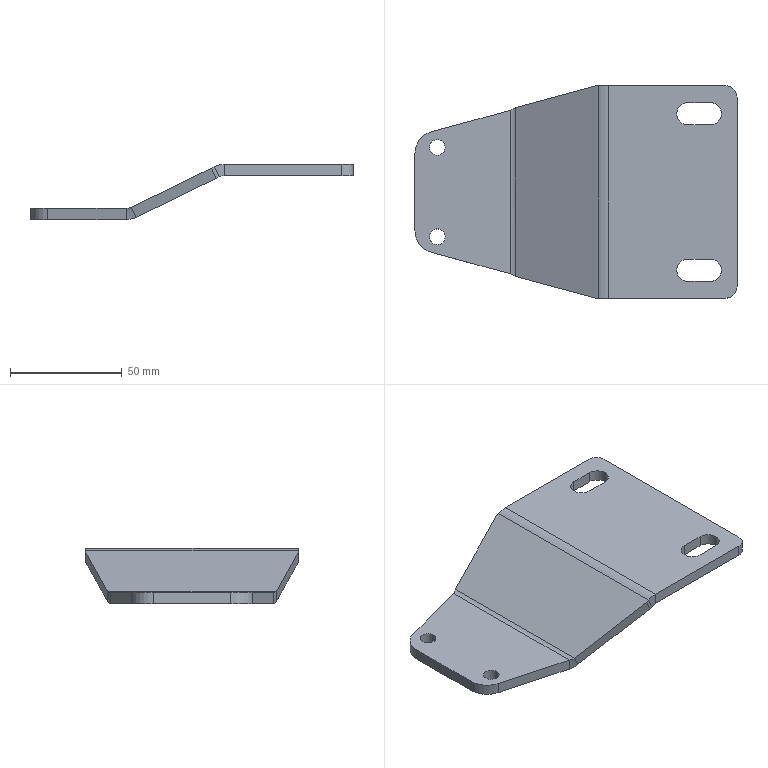Part | STEP file | SYL_0392D6J1SYL0380DJ10-1504831 | 1 solid | 44 faces | box 144.153 x 95 x 24.659 mm | volume 58803 mm3 | plane 22 | cylinder 20 | spline 2 | commonest cylinder face diameters 10 x12 7 x4 20 x4
STEP:
#1=CARTESIAN_POINT('',(18.,30.,0.));
#2=VERTEX_POINT('',#1);
#3=CARTESIAN_POINT('',(18.,30.,5.));
#4=VERTEX_POINT('',#3);
#5=CARTESIAN_POINT('',(18.,30.,5.));
#6=DIRECTION('',(0.,0.,1.));
#7=VECTOR('',#6,1000.);
#8=LINE('',#5,#7);
#9=EDGE_CURVE('',#2,#4,#8,.T.);
#10=ORIENTED_EDGE('',*,*,#9,.F.);
#11=CARTESIAN_POINT('',(8.,30.,0.));
#12=VERTEX_POINT('',#11);
#13=CARTESIAN_POINT('',(0.,30.,0.));
#14=DIRECTION('',(1.,0.,0.));
#15=VECTOR('',#14,1000.);
#16=LINE('',#13,#15);
#17=EDGE_CURVE('',#12,#2,#16,.T.);
#18=ORIENTED_EDGE('',*,*,#17,.F.);
#19=CARTESIAN_POINT('',(8.,30.,5.));
#20=VERTEX_POINT('',#19);
#21=CARTESIAN_POINT('',(8.,30.,5.));
#22=DIRECTION('',(0.,0.,1.));
#23=VECTOR('',#22,1000.);
#24=LINE('',#21,#23);
#25=EDGE_CURVE('',#12,#20,#24,.T.);
#26=ORIENTED_EDGE('',*,*,#25,.T.);
#27=CARTESIAN_POINT('',(8.,30.,5.));
#28=DIRECTION('',(1.,0.,0.));
#29=VECTOR('',#28,1000.);
#30=LINE('',#27,#29);
#31=EDGE_CURVE('',#20,#4,#30,.T.);
#32=ORIENTED_EDGE('',*,*,#31,.T.);
#33=EDGE_LOOP('',(#10,#18,#26,#32));
#34=FACE_OUTER_BOUND('',#33,.T.);
#35=CARTESIAN_POINT('',(8.,30.,5.));
#36=DIRECTION('',(0.,-1.,0.));
#37=DIRECTION('',(1.,0.,0.));
#38=AXIS2_PLACEMENT_3D('',#35,#36,#37);
#39=PLANE('',#38);
#40=ADVANCED_FACE('',(#34),#39,.F.);
#41=ORIENTED_EDGE('',*,*,#25,.F.);
#42=CARTESIAN_POINT('',(3.,35.,0.));
#43=VERTEX_POINT('',#42);
#44=CARTESIAN_POINT('',(8.,35.,0.));
#45=DIRECTION('',(0.,0.,-1.));
#46=DIRECTION('',(-1.,0.,0.));
#47=AXIS2_PLACEMENT_3D('',#44,#45,#46);
#48=CIRCLE('',#47,5.);
#49=EDGE_CURVE('',#12,#43,#48,.T.);
#50=ORIENTED_EDGE('',*,*,#49,.T.);
#51=CARTESIAN_POINT('',(3.,35.,5.));
#52=VERTEX_POINT('',#51);
#53=CARTESIAN_POINT('',(3.,35.,5.));
#54=DIRECTION('',(0.,0.,1.));
#55=VECTOR('',#54,1000.);
#56=LINE('',#53,#55);
#57=EDGE_CURVE('',#43,#52,#56,.T.);
#58=ORIENTED_EDGE('',*,*,#57,.T.);
#59=CARTESIAN_POINT('',(8.,35.,5.));
#60=DIRECTION('',(0.,0.,-1.));
#61=DIRECTION('',(0.,-1.,0.));
#62=AXIS2_PLACEMENT_3D('',#59,#60,#61);
#63=CIRCLE('',#62,5.);
#64=EDGE_CURVE('',#20,#52,#63,.T.);
#65=ORIENTED_EDGE('',*,*,#64,.F.);
#66=EDGE_LOOP('',(#41,#50,#58,#65));
#67=FACE_OUTER_BOUND('',#66,.T.);
#68=CARTESIAN_POINT('',(8.,35.,5.));
#69=DIRECTION('',(0.,0.,1.));
#70=DIRECTION('',(1.,0.,0.));
#71=AXIS2_PLACEMENT_3D('',#68,#69,#70);
#72=CYLINDRICAL_SURFACE('',#71,5.);
#73=ADVANCED_FACE('',(#67),#72,.F.);
#74=ORIENTED_EDGE('',*,*,#57,.F.);
#75=CARTESIAN_POINT('',(8.,40.,0.));
#76=VERTEX_POINT('',#75);
#77=CARTESIAN_POINT('',(8.,35.,0.));
#78=DIRECTION('',(0.,0.,-1.));
#79=DIRECTION('',(-1.,0.,0.));
#80=AXIS2_PLACEMENT_3D('',#77,#78,#79);
#81=CIRCLE('',#80,5.);
#82=EDGE_CURVE('',#43,#76,#81,.T.);
#83=ORIENTED_EDGE('',*,*,#82,.T.);
#84=CARTESIAN_POINT('',(8.,40.,5.));
#85=VERTEX_POINT('',#84);
#86=CARTESIAN_POINT('',(8.,40.,5.));
#87=DIRECTION('',(0.,0.,1.));
#88=VECTOR('',#87,1000.);
#89=LINE('',#86,#88);
#90=EDGE_CURVE('',#76,#85,#89,.T.);
#91=ORIENTED_EDGE('',*,*,#90,.T.);
#92=CARTESIAN_POINT('',(8.,35.,5.));
#93=DIRECTION('',(0.,0.,-1.));
#94=DIRECTION('',(-1.,0.,0.));
#95=AXIS2_PLACEMENT_3D('',#92,#93,#94);
#96=CIRCLE('',#95,5.);
#97=EDGE_CURVE('',#52,#85,#96,.T.);
#98=ORIENTED_EDGE('',*,*,#97,.F.);
#99=EDGE_LOOP('',(#74,#83,#91,#98));
#100=FACE_OUTER_BOUND('',#99,.T.);
#101=CARTESIAN_POINT('',(8.,35.,5.));
#102=DIRECTION('',(0.,0.,1.));
#103=DIRECTION('',(1.,0.,0.));
#104=AXIS2_PLACEMENT_3D('',#101,#102,#103);
#105=CYLINDRICAL_SURFACE('',#104,5.);
#106=ADVANCED_FACE('',(#100),#105,.F.);
#107=ORIENTED_EDGE('',*,*,#90,.F.);
#108=CARTESIAN_POINT('',(18.,40.,0.));
#109=VERTEX_POINT('',#108);
#110=CARTESIAN_POINT('',(0.,40.,0.));
#111=DIRECTION('',(-1.,0.,0.));
#112=VECTOR('',#111,1000.);
#113=LINE('',#110,#112);
#114=EDGE_CURVE('',#109,#76,#113,.T.);
#115=ORIENTED_EDGE('',*,*,#114,.F.);
#116=CARTESIAN_POINT('',(18.,40.,5.));
#117=VERTEX_POINT('',#116);
#118=CARTESIAN_POINT('',(18.,40.,5.));
#119=DIRECTION('',(0.,0.,1.));
#120=VECTOR('',#119,1000.);
#121=LINE('',#118,#120);
#122=EDGE_CURVE('',#109,#117,#121,.T.);
#123=ORIENTED_EDGE('',*,*,#122,.T.);
#124=CARTESIAN_POINT('',(18.,40.,5.));
#125=DIRECTION('',(-1.,0.,0.));
#126=VECTOR('',#125,1000.);
#127=LINE('',#124,#126);
#128=EDGE_CURVE('',#117,#85,#127,.T.);
#129=ORIENTED_EDGE('',*,*,#128,.T.);
#130=EDGE_LOOP('',(#107,#115,#123,#129));
#131=FACE_OUTER_BOUND('',#130,.T.);
#132=CARTESIAN_POINT('',(18.,40.,5.));
#133=DIRECTION('',(0.,1.,0.));
#134=DIRECTION('',(-1.,0.,0.));
#135=AXIS2_PLACEMENT_3D('',#132,#133,#134);
#136=PLANE('',#135);
#137=ADVANCED_FACE('',(#131),#136,.F.);
#138=ORIENTED_EDGE('',*,*,#122,.F.);
#139=CARTESIAN_POINT('',(23.,35.,0.));
#140=VERTEX_POINT('',#139);
#141=CARTESIAN_POINT('',(18.,35.,0.));
#142=DIRECTION('',(0.,0.,-1.));
#143=DIRECTION('',(-1.,0.,0.));
#144=AXIS2_PLACEMENT_3D('',#141,#142,#143);
#145=CIRCLE('',#144,5.);
#146=EDGE_CURVE('',#109,#140,#145,.T.);
#147=ORIENTED_EDGE('',*,*,#146,.T.);
#148=CARTESIAN_POINT('',(23.,35.,5.));
#149=VERTEX_POINT('',#148);
#150=CARTESIAN_POINT('',(23.,35.,5.));
#151=DIRECTION('',(0.,0.,1.));
#152=VECTOR('',#151,1000.);
#153=LINE('',#150,#152);
#154=EDGE_CURVE('',#140,#149,#153,.T.);
#155=ORIENTED_EDGE('',*,*,#154,.T.);
#156=CARTESIAN_POINT('',(18.,35.,5.));
#157=DIRECTION('',(0.,0.,-1.));
#158=DIRECTION('',(0.,1.,0.));
#159=AXIS2_PLACEMENT_3D('',#156,#157,#158);
#160=CIRCLE('',#159,5.);
#161=EDGE_CURVE('',#117,#149,#160,.T.);
#162=ORIENTED_EDGE('',*,*,#161,.F.);
#163=EDGE_LOOP('',(#138,#147,#155,#162));
#164=FACE_OUTER_BOUND('',#163,.T.);
#165=CARTESIAN_POINT('',(18.,35.,5.));
#166=DIRECTION('',(0.,0.,1.));
#167=DIRECTION('',(1.,0.,0.));
#168=AXIS2_PLACEMENT_3D('',#165,#166,#167);
#169=CYLINDRICAL_SURFACE('',#168,5.);
#170=ADVANCED_FACE('',(#164),#169,.F.);
#171=CARTESIAN_POINT('',(8.,-40.,0.));
#172=VERTEX_POINT('',#171);
#173=CARTESIAN_POINT('',(8.,-40.,5.));
#174=VERTEX_POINT('',#173);
#175=CARTESIAN_POINT('',(8.,-40.,5.));
#176=DIRECTION('',(0.,0.,1.));
#177=VECTOR('',#176,1000.);
#178=LINE('',#175,#177);
#179=EDGE_CURVE('',#172,#174,#178,.T.);
#180=ORIENTED_EDGE('',*,*,#179,.F.);
#181=CARTESIAN_POINT('',(3.,-35.,0.));
#182=VERTEX_POINT('',#181);
#183=CARTESIAN_POINT('',(8.,-35.,0.));
#184=DIRECTION('',(0.,0.,-1.));
#185=DIRECTION('',(-1.,0.,0.));
#186=AXIS2_PLACEMENT_3D('',#183,#184,#185);
#187=CIRCLE('',#186,5.);
#188=EDGE_CURVE('',#172,#182,#187,.T.);
#189=ORIENTED_EDGE('',*,*,#188,.T.);
#190=CARTESIAN_POINT('',(3.,-35.,5.));
#191=VERTEX_POINT('',#190);
#192=CARTESIAN_POINT('',(3.,-35.,5.));
#193=DIRECTION('',(0.,0.,1.));
#194=VECTOR('',#193,1000.);
#195=LINE('',#192,#194);
#196=EDGE_CURVE('',#182,#191,#195,.T.);
#197=ORIENTED_EDGE('',*,*,#196,.T.);
#198=CARTESIAN_POINT('',(8.,-35.,5.));
#199=DIRECTION('',(0.,0.,-1.));
#200=DIRECTION('',(0.,-1.,0.));
#201=AXIS2_PLACEMENT_3D('',#198,#199,#200);
#202=CIRCLE('',#201,5.);
#203=EDGE_CURVE('',#174,#191,#202,.T.);
#204=ORIENTED_EDGE('',*,*,#203,.F.);
#205=EDGE_LOOP('',(#180,#189,#197,#204));
#206=FACE_OUTER_BOUND('',#205,.T.);
#207=CARTESIAN_POINT('',(8.,-35.,5.));
#208=DIRECTION('',(0.,0.,1.));
#209=DIRECTION('',(1.,0.,0.));
#210=AXIS2_PLACEMENT_3D('',#207,#208,#209);
#211=CYLINDRICAL_SURFACE('',#210,5.);
#212=ADVANCED_FACE('',(#206),#211,.F.);
#213=ORIENTED_EDGE('',*,*,#196,.F.);
#214=CARTESIAN_POINT('',(8.,-30.,0.));
#215=VERTEX_POINT('',#214);
#216=CARTESIAN_POINT('',(8.,-35.,0.));
#217=DIRECTION('',(0.,0.,-1.));
#218=DIRECTION('',(-1.,0.,0.));
#219=AXIS2_PLACEMENT_3D('',#216,#217,#218);
#220=CIRCLE('',#219,5.);
#221=EDGE_CURVE('',#182,#215,#220,.T.);
#222=ORIENTED_EDGE('',*,*,#221,.T.);
#223=CARTESIAN_POINT('',(8.,-30.,5.));
#224=VERTEX_POINT('',#223);
#225=CARTESIAN_POINT('',(8.,-30.,5.));
#226=DIRECTION('',(0.,0.,1.));
#227=VECTOR('',#226,1000.);
#228=LINE('',#225,#227);
#229=EDGE_CURVE('',#215,#224,#228,.T.);
#230=ORIENTED_EDGE('',*,*,#229,.T.);
#231=CARTESIAN_POINT('',(8.,-35.,5.));
#232=DIRECTION('',(0.,0.,-1.));
#233=DIRECTION('',(-1.,0.,0.));
#234=AXIS2_PLACEMENT_3D('',#231,#232,#233);
#235=CIRCLE('',#234,5.);
#236=EDGE_CURVE('',#191,#224,#235,.T.);
#237=ORIENTED_EDGE('',*,*,#236,.F.);
#238=EDGE_LOOP('',(#213,#222,#230,#237));
#239=FACE_OUTER_BOUND('',#238,.T.);
#240=CARTESIAN_POINT('',(8.,-35.,5.));
#241=DIRECTION('',(0.,0.,1.));
#242=DIRECTION('',(1.,0.,0.));
#243=AXIS2_PLACEMENT_3D('',#240,#241,#242);
#244=CYLINDRICAL_SURFACE('',#243,5.);
#245=ADVANCED_FACE('',(#239),#244,.F.);
#246=ORIENTED_EDGE('',*,*,#229,.F.);
#247=CARTESIAN_POINT('',(18.,-30.,0.));
#248=VERTEX_POINT('',#247);
#249=CARTESIAN_POINT('',(0.,-30.,0.));
#250=DIRECTION('',(-1.,0.,0.));
#251=VECTOR('',#250,1000.);
#252=LINE('',#249,#251);
#253=EDGE_CURVE('',#248,#215,#252,.T.);
#254=ORIENTED_EDGE('',*,*,#253,.F.);
#255=CARTESIAN_POINT('',(18.,-30.,5.));
#256=VERTEX_POINT('',#255);
#257=CARTESIAN_POINT('',(18.,-30.,5.));
#258=DIRECTION('',(0.,0.,1.));
#259=VECTOR('',#258,1000.);
#260=LINE('',#257,#259);
#261=EDGE_CURVE('',#248,#256,#260,.T.);
#262=ORIENTED_EDGE('',*,*,#261,.T.);
#263=CARTESIAN_POINT('',(18.,-30.,5.));
#264=DIRECTION('',(-1.,0.,0.));
#265=VECTOR('',#264,1000.);
#266=LINE('',#263,#265);
#267=EDGE_CURVE('',#256,#224,#266,.T.);
#268=ORIENTED_EDGE('',*,*,#267,.T.);
#269=EDGE_LOOP('',(#246,#254,#262,#268));
#270=FACE_OUTER_BOUND('',#269,.T.);
#271=CARTESIAN_POINT('',(18.,-30.,5.));
#272=DIRECTION('',(0.,1.,0.));
#273=DIRECTION('',(-1.,0.,0.));
#274=AXIS2_PLACEMENT_3D('',#271,#272,#273);
#275=PLANE('',#274);
#276=ADVANCED_FACE('',(#270),#275,.F.);
#277=ORIENTED_EDGE('',*,*,#261,.F.);
#278=CARTESIAN_POINT('',(23.,-35.,0.));
#279=VERTEX_POINT('',#278);
#280=CARTESIAN_POINT('',(18.,-35.,0.));
#281=DIRECTION('',(0.,0.,-1.));
#282=DIRECTION('',(-1.,0.,0.));
#283=AXIS2_PLACEMENT_3D('',#280,#281,#282);
#284=CIRCLE('',#283,5.);
#285=EDGE_CURVE('',#248,#279,#284,.T.);
#286=ORIENTED_EDGE('',*,*,#285,.T.);
#287=CARTESIAN_POINT('',(23.,-35.,5.));
#288=VERTEX_POINT('',#287);
#289=CARTESIAN_POINT('',(23.,-35.,5.));
#290=DIRECTION('',(0.,0.,1.));
#291=VECTOR('',#290,1000.);
#292=LINE('',#289,#291);
#293=EDGE_CURVE('',#279,#288,#292,.T.);
#294=ORIENTED_EDGE('',*,*,#293,.T.);
#295=CARTESIAN_POINT('',(18.,-35.,5.));
#296=DIRECTION('',(0.,0.,-1.));
#297=DIRECTION('',(0.,1.,0.));
#298=AXIS2_PLACEMENT_3D('',#295,#296,#297);
#299=CIRCLE('',#298,5.);
#300=EDGE_CURVE('',#256,#288,#299,.T.);
#301=ORIENTED_EDGE('',*,*,#300,.F.);
#302=EDGE_LOOP('',(#277,#286,#294,#301));
#303=FACE_OUTER_BOUND('',#302,.T.);
#304=CARTESIAN_POINT('',(18.,-35.,5.));
#305=DIRECTION('',(0.,0.,1.));
#306=DIRECTION('',(1.,0.,0.));
#307=AXIS2_PLACEMENT_3D('',#304,#305,#306);
#308=CYLINDRICAL_SURFACE('',#307,5.);
#309=ADVANCED_FACE('',(#303),#308,.F.);
#310=ORIENTED_EDGE('',*,*,#293,.F.);
#311=CARTESIAN_POINT('',(18.,-40.,0.));
#312=VERTEX_POINT('',#311);
#313=CARTESIAN_POINT('',(18.,-35.,0.));
#314=DIRECTION('',(0.,0.,-1.));
#315=DIRECTION('',(-1.,0.,0.));
#316=AXIS2_PLACEMENT_3D('',#313,#314,#315);
#317=CIRCLE('',#316,5.);
#318=EDGE_CURVE('',#279,#312,#317,.T.);
#319=ORIENTED_EDGE('',*,*,#318,.T.);
#320=CARTESIAN_POINT('',(18.,-40.,5.));
#321=VERTEX_POINT('',#320);
#322=CARTESIAN_POINT('',(18.,-40.,5.));
#323=DIRECTION('',(0.,0.,1.));
#324=VECTOR('',#323,1000.);
#325=LINE('',#322,#324);
#326=EDGE_CURVE('',#312,#321,#325,.T.);
#327=ORIENTED_EDGE('',*,*,#326,.T.);
#328=CARTESIAN_POINT('',(18.,-35.,5.));
#329=DIRECTION('',(0.,0.,-1.));
#330=DIRECTION('',(1.,0.,0.));
#331=AXIS2_PLACEMENT_3D('',#328,#329,#330);
#332=CIRCLE('',#331,5.);
#333=EDGE_CURVE('',#288,#321,#332,.T.);
#334=ORIENTED_EDGE('',*,*,#333,.F.);
#335=EDGE_LOOP('',(#310,#319,#327,#334));
#336=FACE_OUTER_BOUND('',#335,.T.);
#337=CARTESIAN_POINT('',(18.,-35.,5.));
#338=DIRECTION('',(0.,0.,1.));
#339=DIRECTION('',(1.,0.,0.));
#340=AXIS2_PLACEMENT_3D('',#337,#338,#339);
#341=CYLINDRICAL_SURFACE('',#340,5.);
#342=ADVANCED_FACE('',(#336),#341,.F.);
#343=CARTESIAN_POINT('',(-100.653,-20.,-19.659));
#344=VERTEX_POINT('',#343);
#345=CARTESIAN_POINT('',(-100.653,-20.,-14.659));
#346=VERTEX_POINT('',#345);
#347=CARTESIAN_POINT('',(-100.653,-20.,-14.659));
#348=DIRECTION('',(0.,0.,1.));
#349=VECTOR('',#348,1000.);
#350=LINE('',#347,#349);
#351=EDGE_CURVE('',#344,#346,#350,.T.);
#352=ORIENTED_EDGE('',*,*,#351,.F.);
#353=CARTESIAN_POINT('',(-107.653,-20.,-19.659));
#354=VERTEX_POINT('',#353);
#355=CARTESIAN_POINT('',(-104.153,-20.,-19.659));
#356=DIRECTION('',(0.,0.,-1.));
#357=DIRECTION('',(-1.,0.,0.));
#358=AXIS2_PLACEMENT_3D('',#355,#356,#357);
#359=CIRCLE('',#358,3.5);
#360=EDGE_CURVE('',#344,#354,#359,.T.);
#361=ORIENTED_EDGE('',*,*,#360,.T.);
#362=CARTESIAN_POINT('',(-107.653,-20.,-14.659));
#363=VERTEX_POINT('',#362);
#364=CARTESIAN_POINT('',(-107.653,-20.,-14.659));
#365=DIRECTION('',(0.,0.,1.));
#366=VECTOR('',#365,1000.);
#367=LINE('',#364,#366);
#368=EDGE_CURVE('',#354,#363,#367,.T.);
#369=ORIENTED_EDGE('',*,*,#368,.T.);
#370=CARTESIAN_POINT('',(-104.153,-20.,-14.659));
#371=DIRECTION('',(0.,0.,-1.));
#372=DIRECTION('',(1.,0.,0.));
#373=AXIS2_PLACEMENT_3D('',#370,#371,#372);
#374=CIRCLE('',#373,3.5);
#375=EDGE_CURVE('',#346,#363,#374,.T.);
#376=ORIENTED_EDGE('',*,*,#375,.F.);
#377=EDGE_LOOP('',(#352,#361,#369,#376));
#378=FACE_OUTER_BOUND('',#377,.T.);
#379=CARTESIAN_POINT('',(-104.153,-20.,-14.659));
#380=DIRECTION('',(0.,0.,-1.));
#381=DIRECTION('',(-1.,0.,0.));
#382=AXIS2_PLACEMENT_3D('',#379,#380,#381);
#383=CYLINDRICAL_SURFACE('',#382,3.5);
#384=ADVANCED_FACE('',(#378),#383,.F.);
#385=CARTESIAN_POINT('',(-100.653,20.,-19.659));
#386=VERTEX_POINT('',#385);
#387=CARTESIAN_POINT('',(-100.653,20.,-14.659));
#388=VERTEX_POINT('',#387);
#389=CARTESIAN_POINT('',(-100.653,20.,-14.659));
#390=DIRECTION('',(0.,0.,1.));
#391=VECTOR('',#390,1000.);
#392=LINE('',#389,#391);
#393=EDGE_CURVE('',#386,#388,#392,.T.);
#394=ORIENTED_EDGE('',*,*,#393,.F.);
#395=CARTESIAN_POINT('',(-107.653,20.,-19.659));
#396=VERTEX_POINT('',#395);
#397=CARTESIAN_POINT('',(-104.153,20.,-19.659));
#398=DIRECTION('',(0.,0.,-1.));
#399=DIRECTION('',(-1.,0.,0.));
#400=AXIS2_PLACEMENT_3D('',#397,#398,#399);
#401=CIRCLE('',#400,3.5);
#402=EDGE_CURVE('',#386,#396,#401,.T.);
#403=ORIENTED_EDGE('',*,*,#402,.T.);
#404=CARTESIAN_POINT('',(-107.653,20.,-14.659));
#405=VERTEX_POINT('',#404);
#406=CARTESIAN_POINT('',(-107.653,20.,-14.659));
#407=DIRECTION('',(0.,0.,1.));
#408=VECTOR('',#407,1000.);
#409=LINE('',#406,#408);
#410=EDGE_CURVE('',#396,#405,#409,.T.);
#411=ORIENTED_EDGE('',*,*,#410,.T.);
#412=CARTESIAN_POINT('',(-104.153,20.,-14.659));
#413=DIRECTION('',(0.,0.,-1.));
#414=DIRECTION('',(1.,0.,0.));
#415=AXIS2_PLACEMENT_3D('',#412,#413,#414);
#416=CIRCLE('',#415,3.5);
#417=EDGE_CURVE('',#388,#405,#416,.T.);
#418=ORIENTED_EDGE('',*,*,#417,.F.);
#419=EDGE_LOOP('',(#394,#403,#411,#418));
#420=FACE_OUTER_BOUND('',#419,.T.);
#421=CARTESIAN_POINT('',(-104.153,20.,-14.659));
#422=DIRECTION('',(0.,0.,-1.));
#423=DIRECTION('',(-1.,0.,0.));
#424=AXIS2_PLACEMENT_3D('',#421,#422,#423);
#425=CYLINDRICAL_SURFACE('',#424,3.5);
#426=ADVANCED_FACE('',(#420),#425,.F.);
#427=CARTESIAN_POINT('',(-106.769,27.002,-19.659));
#428=VERTEX_POINT('',#427);
#429=CARTESIAN_POINT('',(-106.769,27.002,-14.659));
#430=VERTEX_POINT('',#429);
#431=CARTESIAN_POINT('',(-106.769,27.002,-14.659));
#432=DIRECTION('',(0.,0.,1.));
#433=VECTOR('',#432,1000.);
#434=LINE('',#431,#433);
#435=EDGE_CURVE('',#428,#430,#434,.T.);
#436=ORIENTED_EDGE('',*,*,#435,.F.);
#437=CARTESIAN_POINT('',(-114.153,17.35,-19.659));
#438=VERTEX_POINT('',#437);
#439=CARTESIAN_POINT('',(-104.153,17.35,-19.659));
#440=DIRECTION('',(0.,0.,1.));
#441=DIRECTION('',(1.,0.,0.));
#442=AXIS2_PLACEMENT_3D('',#439,#440,#441);
#443=CIRCLE('',#442,10.);
#444=EDGE_CURVE('',#428,#438,#443,.T.);
#445=ORIENTED_EDGE('',*,*,#444,.T.);
#446=CARTESIAN_POINT('',(-114.153,17.35,-14.659));
#447=VERTEX_POINT('',#446);
#448=CARTESIAN_POINT('',(-114.153,17.35,-14.659));
#449=DIRECTION('',(0.,0.,1.));
#450=VECTOR('',#449,1000.);
#451=LINE('',#448,#450);
#452=EDGE_CURVE('',#438,#447,#451,.T.);
#453=ORIENTED_EDGE('',*,*,#452,.T.);
#454=CARTESIAN_POINT('',(-104.153,17.35,-14.659));
#455=DIRECTION('',(0.,0.,1.));
#456=DIRECTION('',(-0.2616,0.9652,0.));
#457=AXIS2_PLACEMENT_3D('',#454,#455,#456);
#458=CIRCLE('',#457,10.);
#459=EDGE_CURVE('',#430,#447,#458,.T.);
#460=ORIENTED_EDGE('',*,*,#459,.F.);
#461=EDGE_LOOP('',(#436,#445,#453,#460));
#462=FACE_OUTER_BOUND('',#461,.T.);
#463=CARTESIAN_POINT('',(-104.153,17.35,-14.659));
#464=DIRECTION('',(0.,0.,-1.));
#465=DIRECTION('',(-1.,0.,0.));
#466=AXIS2_PLACEMENT_3D('',#463,#464,#465);
#467=CYLINDRICAL_SURFACE('',#466,10.);
#468=ADVANCED_FACE('',(#462),#467,.T.);
#469=ORIENTED_EDGE('',*,*,#452,.F.);
#470=CARTESIAN_POINT('',(-114.153,-17.35,-19.659));
#471=VERTEX_POINT('',#470);
#472=CARTESIAN_POINT('',(-114.153,-47.5,-19.659));
#473=DIRECTION('',(0.,-1.,0.));
#474=VECTOR('',#473,1000.);
#475=LINE('',#472,#474);
#476=EDGE_CURVE('',#438,#471,#475,.T.);
#477=ORIENTED_EDGE('',*,*,#476,.T.);
#478=CARTESIAN_POINT('',(-114.153,-17.35,-14.659));
#479=VERTEX_POINT('',#478);
#480=CARTESIAN_POINT('',(-114.153,-17.35,-14.659));
#481=DIRECTION('',(0.,0.,1.));
#482=VECTOR('',#481,1000.);
#483=LINE('',#480,#482);
#484=EDGE_CURVE('',#471,#479,#483,.T.);
#485=ORIENTED_EDGE('',*,*,#484,.T.);
#486=CARTESIAN_POINT('',(-114.153,17.35,-14.659));
#487=DIRECTION('',(0.,-1.,0.));
#488=VECTOR('',#487,1000.);
#489=LINE('',#486,#488);
#490=EDGE_CURVE('',#447,#479,#489,.T.);
#491=ORIENTED_EDGE('',*,*,#490,.F.);
#492=EDGE_LOOP('',(#469,#477,#485,#491));
#493=FACE_OUTER_BOUND('',#492,.T.);
#494=CARTESIAN_POINT('',(-114.153,17.35,-14.659));
#495=DIRECTION('',(1.,0.,0.));
#496=DIRECTION('',(0.,-1.,0.));
#497=AXIS2_PLACEMENT_3D('',#494,#495,#496);
#498=PLANE('',#497);
#499=ADVANCED_FACE('',(#493),#498,.F.);
#500=ORIENTED_EDGE('',*,*,#484,.F.);
#501=CARTESIAN_POINT('',(-106.769,-27.002,-19.659));
#502=VERTEX_POINT('',#501);
#503=CARTESIAN_POINT('',(-104.153,-17.35,-19.659));
#504=DIRECTION('',(0.,0.,1.));
#505=DIRECTION('',(1.,0.,0.));
#506=AXIS2_PLACEMENT_3D('',#503,#504,#505);
#507=CIRCLE('',#506,10.);
#508=EDGE_CURVE('',#471,#502,#507,.T.);
#509=ORIENTED_EDGE('',*,*,#508,.T.);
#510=CARTESIAN_POINT('',(-106.769,-27.002,-14.659));
#511=VERTEX_POINT('',#510);
#512=CARTESIAN_POINT('',(-106.769,-27.002,-14.659));
#513=DIRECTION('',(0.,0.,1.));
#514=VECTOR('',#513,1000.);
#515=LINE('',#512,#514);
#516=EDGE_CURVE('',#502,#511,#515,.T.);
#517=ORIENTED_EDGE('',*,*,#516,.T.);
#518=CARTESIAN_POINT('',(-104.153,-17.35,-14.659));
#519=DIRECTION('',(0.,0.,1.));
#520=DIRECTION('',(-1.,0.,0.));
#521=AXIS2_PLACEMENT_3D('',#518,#519,#520);
#522=CIRCLE('',#521,10.);
#523=EDGE_CURVE('',#479,#511,#522,.T.);
#524=ORIENTED_EDGE('',*,*,#523,.F.);
#525=EDGE_LOOP('',(#500,#509,#517,#524));
#526=FACE_OUTER_BOUND('',#525,.T.);
#527=CARTESIAN_POINT('',(-104.153,-17.35,-14.659));
#528=DIRECTION('',(0.,0.,-1.));
#529=DIRECTION('',(-1.,0.,0.));
#530=AXIS2_PLACEMENT_3D('',#527,#528,#529);
#531=CYLINDRICAL_SURFACE('',#530,10.);
#532=ADVANCED_FACE('',(#526),#531,.T.);
#533=ORIENTED_EDGE('',*,*,#516,.F.);
#534=CARTESIAN_POINT('',(-71.461,-36.573,-19.659));
#535=VERTEX_POINT('',#534);
#536=CARTESIAN_POINT('',(-106.769,-27.002,-19.659));
#537=DIRECTION('',(0.9652,-0.2616,0.));
#538=VECTOR('',#537,1000.);
#539=LINE('',#536,#538);
#540=EDGE_CURVE('',#502,#535,#539,.T.);
#541=ORIENTED_EDGE('',*,*,#540,.T.);
#542=CARTESIAN_POINT('',(-71.461,-36.573,-14.659));
#543=VERTEX_POINT('',#542);
#544=CARTESIAN_POINT('',(-71.461,-36.573,-19.659));
#545=CARTESIAN_POINT('',(-71.461,-36.573,-17.992));
#546=CARTESIAN_POINT('',(-71.461,-36.573,-16.326));
#547=CARTESIAN_POINT('',(-71.461,-36.573,-14.659));
#548=B_SPLINE_CURVE_WITH_KNOTS('',3,(#544,#545,#546,#547),.UNSPECIFIED.,.F.,.F.,(4,4),(0.,1.),.UNSPECIFIED.);
#549=EDGE_CURVE('',#535,#543,#548,.T.);
#550=ORIENTED_EDGE('',*,*,#549,.T.);
#551=CARTESIAN_POINT('',(-106.769,-27.002,-14.659));
#552=DIRECTION('',(0.9652,-0.2616,0.));
#553=VECTOR('',#552,1000.);
#554=LINE('',#551,#553);
#555=EDGE_CURVE('',#511,#543,#554,.T.);
#556=ORIENTED_EDGE('',*,*,#555,.F.);
#557=EDGE_LOOP('',(#533,#541,#550,#556));
#558=FACE_OUTER_BOUND('',#557,.T.);
#559=CARTESIAN_POINT('',(-106.769,-27.002,-14.659));
#560=DIRECTION('',(0.2616,0.9652,0.));
#561=DIRECTION('',(0.9652,-0.2616,0.));
#562=AXIS2_PLACEMENT_3D('',#559,#560,#561);
#563=PLANE('',#562);
#564=ADVANCED_FACE('',(#558),#563,.F.);
#565=ORIENTED_EDGE('',*,*,#549,.F.);
#566=CARTESIAN_POINT('',(-67.078,-37.761,-18.647));
#567=VERTEX_POINT('',#566);
#568=CARTESIAN_POINT('',(-71.461,-36.573,-19.659));
#569=CARTESIAN_POINT('',(-70.957,-36.71,-19.659));
#570=CARTESIAN_POINT('',(-70.516,-36.829,-19.622));
#571=CARTESIAN_POINT('',(-69.951,-36.982,-19.546));
#572=CARTESIAN_POINT('',(-69.779,-37.029,-19.518));
#573=CARTESIAN_POINT('',(-69.545,-37.092,-19.474));
#574=CARTESIAN_POINT('',(-69.471,-37.113,-19.459));
#575=CARTESIAN_POINT('',(-69.365,-37.141,-19.437));
#576=CARTESIAN_POINT('',(-69.331,-37.15,-19.43));
#577=CARTESIAN_POINT('',(-69.281,-37.164,-19.419));
#578=CARTESIAN_POINT('',(-69.265,-37.168,-19.415));
#579=CARTESIAN_POINT('',(-69.241,-37.175,-19.409));
#580=CARTESIAN_POINT('',(-69.233,-37.177,-19.408));
#581=CARTESIAN_POINT('',(-69.217,-37.181,-19.404));
#582=CARTESIAN_POINT('',(-69.214,-37.182,-19.403));
#583=CARTESIAN_POINT('',(-68.389,-37.406,-19.212));
#584=CARTESIAN_POINT('',(-67.68,-37.598,-18.941));
#585=CARTESIAN_POINT('',(-67.078,-37.761,-18.647));
#586=B_SPLINE_CURVE_WITH_KNOTS('',3,(#568,#569,#570,#571,#572,#573,#574,#575,#576,#577,#578,#579,#580,#581,#582,#583,#584,#585),.UNSPECIFIED.,.F.,.F.,(4,2,2,2,2,2,2,2,4),(0.,0.25,0.375,0.4375,0.4688,0.4844,0.4922,0.5,1.),.UNSPECIFIED.);
#587=EDGE_CURVE('',#535,#567,#586,.T.);
#588=ORIENTED_EDGE('',*,*,#587,.T.);
#589=CARTESIAN_POINT('',(-69.269,-37.761,-14.153));
#590=VERTEX_POINT('',#589);
#591=CARTESIAN_POINT('',(-67.078,-37.761,-18.647));
#592=CARTESIAN_POINT('',(-69.269,-37.761,-14.153));
#593=B_SPLINE_CURVE_WITH_KNOTS('',1,(#591,#592),.UNSPECIFIED.,.F.,.F.,(2,2),(0.,1.),.UNSPECIFIED.);
#594=EDGE_CURVE('',#567,#590,#593,.T.);
#595=ORIENTED_EDGE('',*,*,#594,.T.);
#596=CARTESIAN_POINT('',(-71.461,-36.573,-14.659));
#597=CARTESIAN_POINT('',(-71.209,-36.71,-14.659));
#598=CARTESIAN_POINT('',(-70.989,-36.829,-14.64));
#599=CARTESIAN_POINT('',(-70.706,-36.982,-14.603));
#600=CARTESIAN_POINT('',(-70.62,-37.029,-14.588));
#601=CARTESIAN_POINT('',(-70.503,-37.092,-14.567));
#602=CARTESIAN_POINT('',(-70.466,-37.113,-14.559));
#603=CARTESIAN_POINT('',(-70.413,-37.141,-14.548));
#604=CARTESIAN_POINT('',(-70.388,-37.155,-14.542));
#605=CARTESIAN_POINT('',(-70.359,-37.171,-14.536));
#606=CARTESIAN_POINT('',(-70.345,-37.178,-14.533));
#607=CARTESIAN_POINT('',(-70.339,-37.181,-14.532));
#608=CARTESIAN_POINT('',(-70.335,-37.183,-14.531));
#609=CARTESIAN_POINT('',(-70.335,-37.184,-14.53));
#610=CARTESIAN_POINT('',(-69.925,-37.406,-14.435));
#611=CARTESIAN_POINT('',(-69.571,-37.598,-14.3));
#612=CARTESIAN_POINT('',(-69.269,-37.761,-14.153));
#613=B_SPLINE_CURVE_WITH_KNOTS('',3,(#596,#597,#598,#599,#600,#601,#602,#603,#604,#605,#606,#607,#608,#609,#610,#611,#612),.UNSPECIFIED.,.F.,.F.,(4,2,2,2,1,1,1,2,2,4),(0.,0.25,0.375,0.4375,0.4688,0.4844,0.4922,0.4961,0.5,1.),.UNSPECIFIED.);
#614=EDGE_CURVE('',#543,#590,#613,.T.);
#615=ORIENTED_EDGE('',*,*,#614,.F.);
#616=EDGE_LOOP('',(#565,#588,#595,#615));
#617=FACE_OUTER_BOUND('',#616,.T.);
#618=CARTESIAN_POINT('',(-71.461,-36.573,-19.659));
#619=CARTESIAN_POINT('',(-70.957,-36.71,-19.659));
#620=CARTESIAN_POINT('',(-70.516,-36.829,-19.622));
#621=CARTESIAN_POINT('',(-69.951,-36.982,-19.546));
#622=CARTESIAN_POINT('',(-69.779,-37.029,-19.518));
#623=CARTESIAN_POINT('',(-69.545,-37.092,-19.474));
#624=CARTESIAN_POINT('',(-69.471,-37.113,-19.459));
#625=CARTESIAN_POINT('',(-69.365,-37.141,-19.437));
#626=CARTESIAN_POINT('',(-69.331,-37.15,-19.43));
#627=CARTESIAN_POINT('',(-69.281,-37.164,-19.419));
#628=CARTESIAN_POINT('',(-69.265,-37.168,-19.415));
#629=CARTESIAN_POINT('',(-69.241,-37.175,-19.409));
#630=CARTESIAN_POINT('',(-69.233,-37.177,-19.408));
#631=CARTESIAN_POINT('',(-69.217,-37.181,-19.404));
#632=CARTESIAN_POINT('',(-69.214,-37.182,-19.403));
#633=CARTESIAN_POINT('',(-68.389,-37.406,-19.212));
#634=CARTESIAN_POINT('',(-67.68,-37.598,-18.941));
#635=CARTESIAN_POINT('',(-67.078,-37.761,-18.647));
#636=CARTESIAN_POINT('',(-71.461,-36.573,-14.659));
#637=CARTESIAN_POINT('',(-71.209,-36.71,-14.659));
#638=CARTESIAN_POINT('',(-70.989,-36.829,-14.64));
#639=CARTESIAN_POINT('',(-70.706,-36.982,-14.603));
#640=CARTESIAN_POINT('',(-70.62,-37.029,-14.588));
#641=CARTESIAN_POINT('',(-70.503,-37.092,-14.567));
#642=CARTESIAN_POINT('',(-70.466,-37.113,-14.559));
#643=CARTESIAN_POINT('',(-70.413,-37.141,-14.548));
#644=CARTESIAN_POINT('',(-70.396,-37.15,-14.544));
#645=CARTESIAN_POINT('',(-70.371,-37.164,-14.539));
#646=CARTESIAN_POINT('',(-70.363,-37.168,-14.537));
#647=CARTESIAN_POINT('',(-70.351,-37.175,-14.534));
#648=CARTESIAN_POINT('',(-70.347,-37.177,-14.533));
#649=CARTESIAN_POINT('',(-70.339,-37.181,-14.531));
#650=CARTESIAN_POINT('',(-70.338,-37.182,-14.531));
#651=CARTESIAN_POINT('',(-69.925,-37.406,-14.435));
#652=CARTESIAN_POINT('',(-69.571,-37.598,-14.3));
#653=CARTESIAN_POINT('',(-69.269,-37.761,-14.153));
#654=B_SPLINE_SURFACE_WITH_KNOTS('',1,3,((#618,#619,#620,#621,#622,#623,#624,#625,#626,#627,#628,#629,#630,#631,#632,#633,#634,#635),(#636,#637,#638,#639,#640,#641,#642,#643,#644,#645,#646,#647,#648,#649,#650,#651,#652,#653)),.UNSPECIFIED.,.F.,.F.,.F.,(2,2),(4,2,2,2,2,2,2,2,4),(0.,1.),(0.,0.25,0.375,0.4375,0.4688,0.4844,0.4922,0.5,1.),.UNSPECIFIED.);
#655=ADVANCED_FACE('',(#617),#654,.F.);
#656=ORIENTED_EDGE('',*,*,#594,.F.);
#657=CARTESIAN_POINT('',(-31.153,-47.5,-1.125));
#658=VERTEX_POINT('',#657);
#659=CARTESIAN_POINT('',(-67.078,-37.761,-18.647));
#660=DIRECTION('',(0.8732,-0.2367,0.4259));
#661=VECTOR('',#660,1000.);
#662=LINE('',#659,#661);
#663=EDGE_CURVE('',#567,#658,#662,.T.);
#664=ORIENTED_EDGE('',*,*,#663,.T.);
#665=CARTESIAN_POINT('',(-33.345,-47.5,3.369));
#666=VERTEX_POINT('',#665);
#667=CARTESIAN_POINT('',(-33.345,-47.5,3.369));
#668=DIRECTION('',(-0.4384,0.,0.8988));
#669=VECTOR('',#668,1000.);
#670=LINE('',#667,#669);
#671=EDGE_CURVE('',#658,#666,#670,.T.);
#672=ORIENTED_EDGE('',*,*,#671,.T.);
#673=CARTESIAN_POINT('',(-69.269,-37.761,-14.153));
#674=DIRECTION('',(0.8732,-0.2367,0.4259));
#675=VECTOR('',#674,1000.);
#676=LINE('',#673,#675);
#677=EDGE_CURVE('',#590,#666,#676,.T.);
#678=ORIENTED_EDGE('',*,*,#677,.F.);
#679=EDGE_LOOP('',(#656,#664,#672,#678));
#680=FACE_OUTER_BOUND('',#679,.T.);
#681=CARTESIAN_POINT('',(-69.269,-37.761,-14.153));
#682=DIRECTION('',(-0.2128,-0.9716,-0.1038));
#683=DIRECTION('',(0.8732,-0.2367,0.4259));
#684=AXIS2_PLACEMENT_3D('',#681,#682,#683);
#685=PLANE('',#684);
#686=ADVANCED_FACE('',(#680),#685,.T.);
#687=ORIENTED_EDGE('',*,*,#671,.F.);
#688=CARTESIAN_POINT('',(-29.883,-47.5,-0.506));
#689=VERTEX_POINT('',#688);
#690=CARTESIAN_POINT('',(-27.808,-47.5,0.506));
#691=DIRECTION('',(-0.8988,0.,-0.4384));
#692=VECTOR('',#691,1000.);
#693=LINE('',#690,#692);
#694=EDGE_CURVE('',#689,#658,#693,.T.);
#695=ORIENTED_EDGE('',*,*,#694,.F.);
#696=CARTESIAN_POINT('',(-32.075,-47.5,3.988));
#697=VERTEX_POINT('',#696);
#698=CARTESIAN_POINT('',(-32.075,-47.5,3.988));
#699=DIRECTION('',(-0.4384,0.,0.8988));
#700=VECTOR('',#699,1000.);
#701=LINE('',#698,#700);
#702=EDGE_CURVE('',#689,#697,#701,.T.);
#703=ORIENTED_EDGE('',*,*,#702,.T.);
#704=CARTESIAN_POINT('',(-32.075,-47.5,3.988));
#705=DIRECTION('',(-0.8988,0.,-0.4384));
#706=VECTOR('',#705,1000.);
#707=LINE('',#704,#706);
#708=EDGE_CURVE('',#697,#666,#707,.T.);
#709=ORIENTED_EDGE('',*,*,#708,.T.);
#710=EDGE_LOOP('',(#687,#695,#703,#709));
#711=FACE_OUTER_BOUND('',#710,.T.);
#712=CARTESIAN_POINT('',(-32.075,-47.5,3.988));
#713=DIRECTION('',(0.,1.,0.));
#714=DIRECTION('',(-0.8988,0.,-0.4384));
#715=AXIS2_PLACEMENT_3D('',#712,#713,#714);
#716=PLANE('',#715);
#717=ADVANCED_FACE('',(#711),#716,.F.);
#718=ORIENTED_EDGE('',*,*,#702,.F.);
#719=CARTESIAN_POINT('',(-27.691,-47.5,0.));
#720=VERTEX_POINT('',#719);
#721=CARTESIAN_POINT('',(-27.691,-47.5,-5.));
#722=DIRECTION('',(0.,-1.,0.));
#723=DIRECTION('',(0.,0.,1.));
#724=AXIS2_PLACEMENT_3D('',#721,#722,#723);
#725=CIRCLE('',#724,5.);
#726=EDGE_CURVE('',#720,#689,#725,.T.);
#727=ORIENTED_EDGE('',*,*,#726,.F.);
#728=CARTESIAN_POINT('',(-27.691,-47.5,5.));
#729=VERTEX_POINT('',#728);
#730=CARTESIAN_POINT('',(-27.691,-47.5,5.));
#731=DIRECTION('',(0.,0.,1.));
#732=VECTOR('',#731,1000.);
#733=LINE('',#730,#732);
#734=EDGE_CURVE('',#720,#729,#733,.T.);
#735=ORIENTED_EDGE('',*,*,#734,.T.);
#736=CARTESIAN_POINT('',(-27.691,-47.5,-5.));
#737=DIRECTION('',(0.,-1.,0.));
#738=DIRECTION('',(0.,0.,1.));
#739=AXIS2_PLACEMENT_3D('',#736,#737,#738);
#740=CIRCLE('',#739,10.);
#741=EDGE_CURVE('',#729,#697,#740,.T.);
#742=ORIENTED_EDGE('',*,*,#741,.T.);
#743=EDGE_LOOP('',(#718,#727,#735,#742));
#744=FACE_OUTER_BOUND('',#743,.T.);
#745=CARTESIAN_POINT('',(-27.691,-47.5,-5.));
#746=DIRECTION('',(0.,1.,0.));
#747=DIRECTION('',(0.,0.,1.));
#748=AXIS2_PLACEMENT_3D('',#745,#746,#747);
#749=PLANE('',#748);
#750=ADVANCED_FACE('',(#744),#749,.F.);
#751=ORIENTED_EDGE('',*,*,#734,.F.);
#752=CARTESIAN_POINT('',(25.,-47.5,0.));
#753=VERTEX_POINT('',#752);
#754=CARTESIAN_POINT('',(0.,-47.5,0.));
#755=DIRECTION('',(-1.,0.,0.));
#756=VECTOR('',#755,1000.);
#757=LINE('',#754,#756);
#758=EDGE_CURVE('',#753,#720,#757,.T.);
#759=ORIENTED_EDGE('',*,*,#758,.F.);
#760=CARTESIAN_POINT('',(25.,-47.5,5.));
#761=VERTEX_POINT('',#760);
#762=CARTESIAN_POINT('',(25.,-47.5,5.));
#763=DIRECTION('',(0.,0.,1.));
#764=VECTOR('',#763,1000.);
#765=LINE('',#762,#764);
#766=EDGE_CURVE('',#753,#761,#765,.T.);
#767=ORIENTED_EDGE('',*,*,#766,.T.);
#768=CARTESIAN_POINT('',(25.,-47.5,5.));
#769=DIRECTION('',(-1.,0.,0.));
#770=VECTOR('',#769,1000.);
#771=LINE('',#768,#770);
#772=EDGE_CURVE('',#761,#729,#771,.T.);
#773=ORIENTED_EDGE('',*,*,#772,.T.);
#774=EDGE_LOOP('',(#751,#759,#767,#773));
#775=FACE_OUTER_BOUND('',#774,.T.);
#776=CARTESIAN_POINT('',(25.,-47.5,5.));
#777=DIRECTION('',(0.,1.,0.));
#778=DIRECTION('',(-1.,0.,0.));
#779=AXIS2_PLACEMENT_3D('',#776,#777,#778);
#780=PLANE('',#779);
#781=ADVANCED_FACE('',(#775),#780,.F.);
#782=ORIENTED_EDGE('',*,*,#766,.F.);
#783=CARTESIAN_POINT('',(30.,-42.5,0.));
#784=VERTEX_POINT('',#783);
#785=CARTESIAN_POINT('',(25.,-42.5,0.));
#786=DIRECTION('',(0.,0.,1.));
#787=DIRECTION('',(1.,0.,0.));
#788=AXIS2_PLACEMENT_3D('',#785,#786,#787);
#789=CIRCLE('',#788,5.);
#790=EDGE_CURVE('',#753,#784,#789,.T.);
#791=ORIENTED_EDGE('',*,*,#790,.T.);
#792=CARTESIAN_POINT('',(30.,-42.5,5.));
#793=VERTEX_POINT('',#792);
#794=CARTESIAN_POINT('',(30.,-42.5,5.));
#795=DIRECTION('',(0.,0.,1.));
#796=VECTOR('',#795,1000.);
#797=LINE('',#794,#796);
#798=EDGE_CURVE('',#784,#793,#797,.T.);
#799=ORIENTED_EDGE('',*,*,#798,.T.);
#800=CARTESIAN_POINT('',(25.,-42.5,5.));
#801=DIRECTION('',(0.,0.,1.));
#802=DIRECTION('',(0.,-1.,0.));
#803=AXIS2_PLACEMENT_3D('',#800,#801,#802);
#804=CIRCLE('',#803,5.);
#805=EDGE_CURVE('',#761,#793,#804,.T.);
#806=ORIENTED_EDGE('',*,*,#805,.F.);
#807=EDGE_LOOP('',(#782,#791,#799,#806));
#808=FACE_OUTER_BOUND('',#807,.T.);
#809=CARTESIAN_POINT('',(25.,-42.5,5.));
#810=DIRECTION('',(0.,0.,1.));
#811=DIRECTION('',(1.,0.,0.));
#812=AXIS2_PLACEMENT_3D('',#809,#810,#811);
#813=CYLINDRICAL_SURFACE('',#812,5.);
#814=ADVANCED_FACE('',(#808),#813,.T.);
#815=ORIENTED_EDGE('',*,*,#798,.F.);
#816=CARTESIAN_POINT('',(30.,42.5,0.));
#817=VERTEX_POINT('',#816);
#818=CARTESIAN_POINT('',(30.,0.,0.));
#819=DIRECTION('',(0.,-1.,0.));
#820=VECTOR('',#819,1000.);
#821=LINE('',#818,#820);
#822=EDGE_CURVE('',#817,#784,#821,.T.);
#823=ORIENTED_EDGE('',*,*,#822,.F.);
#824=CARTESIAN_POINT('',(30.,42.5,5.));
#825=VERTEX_POINT('',#824);
#826=CARTESIAN_POINT('',(30.,42.5,5.));
#827=DIRECTION('',(0.,0.,1.));
#828=VECTOR('',#827,1000.);
#829=LINE('',#826,#828);
#830=EDGE_CURVE('',#817,#825,#829,.T.);
#831=ORIENTED_EDGE('',*,*,#830,.T.);
#832=CARTESIAN_POINT('',(30.,42.5,5.));
#833=DIRECTION('',(0.,-1.,0.));
#834=VECTOR('',#833,1000.);
#835=LINE('',#832,#834);
#836=EDGE_CURVE('',#825,#793,#835,.T.);
#837=ORIENTED_EDGE('',*,*,#836,.T.);
#838=EDGE_LOOP('',(#815,#823,#831,#837));
#839=FACE_OUTER_BOUND('',#838,.T.);
#840=CARTESIAN_POINT('',(30.,42.5,5.));
#841=DIRECTION('',(-1.,0.,0.));
#842=DIRECTION('',(0.,-1.,0.));
#843=AXIS2_PLACEMENT_3D('',#840,#841,#842);
#844=PLANE('',#843);
#845=ADVANCED_FACE('',(#839),#844,.F.);
#846=ORIENTED_EDGE('',*,*,#830,.F.);
#847=CARTESIAN_POINT('',(25.,47.5,0.));
#848=VERTEX_POINT('',#847);
#849=CARTESIAN_POINT('',(25.,42.5,0.));
#850=DIRECTION('',(0.,0.,1.));
#851=DIRECTION('',(1.,0.,0.));
#852=AXIS2_PLACEMENT_3D('',#849,#850,#851);
#853=CIRCLE('',#852,5.);
#854=EDGE_CURVE('',#817,#848,#853,.T.);
#855=ORIENTED_EDGE('',*,*,#854,.T.);
#856=CARTESIAN_POINT('',(25.,47.5,5.));
#857=VERTEX_POINT('',#856);
#858=CARTESIAN_POINT('',(25.,47.5,5.));
#859=DIRECTION('',(0.,0.,1.));
#860=VECTOR('',#859,1000.);
#861=LINE('',#858,#860);
#862=EDGE_CURVE('',#848,#857,#861,.T.);
#863=ORIENTED_EDGE('',*,*,#862,.T.);
#864=CARTESIAN_POINT('',(25.,42.5,5.));
#865=DIRECTION('',(0.,0.,1.));
#866=DIRECTION('',(1.,0.,0.));
#867=AXIS2_PLACEMENT_3D('',#864,#865,#866);
#868=CIRCLE('',#867,5.);
#869=EDGE_CURVE('',#825,#857,#868,.T.);
#870=ORIENTED_EDGE('',*,*,#869,.F.);
#871=EDGE_LOOP('',(#846,#855,#863,#870));
#872=FACE_OUTER_BOUND('',#871,.T.);
#873=CARTESIAN_POINT('',(25.,42.5,5.));
#874=DIRECTION('',(0.,0.,1.));
#875=DIRECTION('',(1.,0.,0.));
#876=AXIS2_PLACEMENT_3D('',#873,#874,#875);
#877=CYLINDRICAL_SURFACE('',#876,5.);
#878=ADVANCED_FACE('',(#872),#877,.T.);
#879=ORIENTED_EDGE('',*,*,#862,.F.);
#880=CARTESIAN_POINT('',(-27.691,47.5,0.));
#881=VERTEX_POINT('',#880);
#882=CARTESIAN_POINT('',(0.,47.5,0.));
#883=DIRECTION('',(1.,0.,0.));
#884=VECTOR('',#883,1000.);
#885=LINE('',#882,#884);
#886=EDGE_CURVE('',#881,#848,#885,.T.);
#887=ORIENTED_EDGE('',*,*,#886,.F.);
#888=CARTESIAN_POINT('',(-27.691,47.5,5.));
#889=VERTEX_POINT('',#888);
#890=CARTESIAN_POINT('',(-27.691,47.5,5.));
#891=DIRECTION('',(0.,0.,1.));
#892=VECTOR('',#891,1000.);
#893=LINE('',#890,#892);
#894=EDGE_CURVE('',#881,#889,#893,.T.);
#895=ORIENTED_EDGE('',*,*,#894,.T.);
#896=CARTESIAN_POINT('',(-27.691,47.5,5.));
#897=DIRECTION('',(1.,0.,0.));
#898=VECTOR('',#897,1000.);
#899=LINE('',#896,#898);
#900=EDGE_CURVE('',#889,#857,#899,.T.);
#901=ORIENTED_EDGE('',*,*,#900,.T.);
#902=EDGE_LOOP('',(#879,#887,#895,#901));
#903=FACE_OUTER_BOUND('',#902,.T.);
#904=CARTESIAN_POINT('',(-27.691,47.5,5.));
#905=DIRECTION('',(0.,-1.,0.));
#906=DIRECTION('',(1.,0.,0.));
#907=AXIS2_PLACEMENT_3D('',#904,#905,#906);
#908=PLANE('',#907);
#909=ADVANCED_FACE('',(#903),#908,.F.);
#910=ORIENTED_EDGE('',*,*,#894,.F.);
#911=CARTESIAN_POINT('',(-29.883,47.5,-0.506));
#912=VERTEX_POINT('',#911);
#913=CARTESIAN_POINT('',(-27.691,47.5,-5.));
#914=DIRECTION('',(0.,1.,0.));
#915=DIRECTION('',(0.,0.,1.));
#916=AXIS2_PLACEMENT_3D('',#913,#914,#915);
#917=CIRCLE('',#916,5.);
#918=EDGE_CURVE('',#912,#881,#917,.T.);
#919=ORIENTED_EDGE('',*,*,#918,.F.);
#920=CARTESIAN_POINT('',(-32.075,47.5,3.988));
#921=VERTEX_POINT('',#920);
#922=CARTESIAN_POINT('',(-32.075,47.5,3.988));
#923=DIRECTION('',(-0.4384,0.,0.8988));
#924=VECTOR('',#923,1000.);
#925=LINE('',#922,#924);
#926=EDGE_CURVE('',#912,#921,#925,.T.);
#927=ORIENTED_EDGE('',*,*,#926,.T.);
#928=CARTESIAN_POINT('',(-27.691,47.5,-5.));
#929=DIRECTION('',(0.,1.,0.));
#930=DIRECTION('',(-0.4384,0.,0.8988));
#931=AXIS2_PLACEMENT_3D('',#928,#929,#930);
#932=CIRCLE('',#931,10.);
#933=EDGE_CURVE('',#921,#889,#932,.T.);
#934=ORIENTED_EDGE('',*,*,#933,.T.);
#935=EDGE_LOOP('',(#910,#919,#927,#934));
#936=FACE_OUTER_BOUND('',#935,.T.);
#937=CARTESIAN_POINT('',(-27.691,47.5,-5.));
#938=DIRECTION('',(0.,-1.,0.));
#939=DIRECTION('',(0.,0.,-1.));
#940=AXIS2_PLACEMENT_3D('',#937,#938,#939);
#941=PLANE('',#940);
#942=ADVANCED_FACE('',(#936),#941,.F.);
#943=ORIENTED_EDGE('',*,*,#926,.F.);
#944=CARTESIAN_POINT('',(-31.153,47.5,-1.125));
#945=VERTEX_POINT('',#944);
#946=CARTESIAN_POINT('',(-27.808,47.5,0.506));
#947=DIRECTION('',(0.8988,0.,0.4384));
#948=VECTOR('',#947,1000.);
#949=LINE('',#946,#948);
#950=EDGE_CURVE('',#945,#912,#949,.T.);
#951=ORIENTED_EDGE('',*,*,#950,.F.);
#952=CARTESIAN_POINT('',(-33.345,47.5,3.369));
#953=VERTEX_POINT('',#952);
#954=CARTESIAN_POINT('',(-33.345,47.5,3.369));
#955=DIRECTION('',(-0.4384,0.,0.8988));
#956=VECTOR('',#955,1000.);
#957=LINE('',#954,#956);
#958=EDGE_CURVE('',#945,#953,#957,.T.);
#959=ORIENTED_EDGE('',*,*,#958,.T.);
#960=CARTESIAN_POINT('',(-33.345,47.5,3.369));
#961=DIRECTION('',(0.8988,0.,0.4384));
#962=VECTOR('',#961,1000.);
#963=LINE('',#960,#962);
#964=EDGE_CURVE('',#953,#921,#963,.T.);
#965=ORIENTED_EDGE('',*,*,#964,.T.);
#966=EDGE_LOOP('',(#943,#951,#959,#965));
#967=FACE_OUTER_BOUND('',#966,.T.);
#968=CARTESIAN_POINT('',(-33.345,47.5,3.369));
#969=DIRECTION('',(0.,-1.,0.));
#970=DIRECTION('',(0.8988,0.,0.4384));
#971=AXIS2_PLACEMENT_3D('',#968,#969,#970);
#972=PLANE('',#971);
#973=ADVANCED_FACE('',(#967),#972,.F.);
#974=ORIENTED_EDGE('',*,*,#958,.F.);
#975=CARTESIAN_POINT('',(-67.078,37.761,-18.647));
#976=VERTEX_POINT('',#975);
#977=CARTESIAN_POINT('',(-67.078,37.761,-18.647));
#978=DIRECTION('',(0.8732,0.2367,0.4259));
#979=VECTOR('',#978,1000.);
#980=LINE('',#977,#979);
#981=EDGE_CURVE('',#976,#945,#980,.T.);
#982=ORIENTED_EDGE('',*,*,#981,.F.);
#983=CARTESIAN_POINT('',(-69.269,37.761,-14.153));
#984=VERTEX_POINT('',#983);
#985=CARTESIAN_POINT('',(-67.078,37.761,-18.647));
#986=CARTESIAN_POINT('',(-67.808,37.761,-17.149));
#987=CARTESIAN_POINT('',(-68.539,37.761,-15.651));
#988=CARTESIAN_POINT('',(-69.269,37.761,-14.153));
#989=B_SPLINE_CURVE_WITH_KNOTS('',3,(#985,#986,#987,#988),.UNSPECIFIED.,.F.,.F.,(4,4),(0.,1.),.UNSPECIFIED.);
#990=EDGE_CURVE('',#976,#984,#989,.T.);
#991=ORIENTED_EDGE('',*,*,#990,.T.);
#992=CARTESIAN_POINT('',(-69.269,37.761,-14.153));
#993=DIRECTION('',(0.8732,0.2367,0.4259));
#994=VECTOR('',#993,1000.);
#995=LINE('',#992,#994);
#996=EDGE_CURVE('',#984,#953,#995,.T.);
#997=ORIENTED_EDGE('',*,*,#996,.T.);
#998=EDGE_LOOP('',(#974,#982,#991,#997));
#999=FACE_OUTER_BOUND('',#998,.T.);
#1000=CARTESIAN_POINT('',(-69.269,37.761,-14.153));
#1001=DIRECTION('',(0.2128,-0.9716,0.1038));
#1002=DIRECTION('',(0.8732,0.2367,0.4259));
#1003=AXIS2_PLACEMENT_3D('',#1000,#1001,#1002);
#1004=PLANE('',#1003);
#1005=ADVANCED_FACE('',(#999),#1004,.F.);
#1006=ORIENTED_EDGE('',*,*,#990,.F.);
#1007=CARTESIAN_POINT('',(-71.461,36.573,-19.659));
#1008=VERTEX_POINT('',#1007);
#1009=CARTESIAN_POINT('',(-67.078,37.761,-18.647));
#1010=CARTESIAN_POINT('',(-67.379,37.68,-18.794));
#1011=CARTESIAN_POINT('',(-67.707,37.591,-18.935));
#1012=CARTESIAN_POINT('',(-68.236,37.447,-19.127));
#1013=CARTESIAN_POINT('',(-68.419,37.398,-19.187));
#1014=CARTESIAN_POINT('',(-68.703,37.321,-19.272));
#1015=CARTESIAN_POINT('',(-68.8,37.294,-19.299));
#1016=CARTESIAN_POINT('',(-68.947,37.255,-19.338));
#1017=CARTESIAN_POINT('',(-68.996,37.241,-19.351));
#1018=CARTESIAN_POINT('',(-69.071,37.221,-19.369));
#1019=CARTESIAN_POINT('',(-69.096,37.214,-19.375));
#1020=CARTESIAN_POINT('',(-69.133,37.204,-19.384));
#1021=CARTESIAN_POINT('',(-69.146,37.201,-19.387));
#1022=CARTESIAN_POINT('',(-69.171,37.194,-19.393));
#1023=CARTESIAN_POINT('',(-69.188,37.189,-19.397));
#1024=CARTESIAN_POINT('',(-69.692,37.053,-19.514));
#1025=CARTESIAN_POINT('',(-70.445,36.849,-19.659));
#1026=CARTESIAN_POINT('',(-71.461,36.573,-19.659));
#1027=B_SPLINE_CURVE_WITH_KNOTS('',3,(#1009,#1010,#1011,#1012,#1013,#1014,#1015,#1016,#1017,#1018,#1019,#1020,#1021,#1022,#1023,#1024,#1025,#1026),.UNSPECIFIED.,.F.,.F.,(4,2,2,2,2,2,2,2,4),(0.,0.25,0.375,0.4375,0.4688,0.4844,0.4922,0.5,1.),.UNSPECIFIED.);
#1028=EDGE_CURVE('',#976,#1008,#1027,.T.);
#1029=ORIENTED_EDGE('',*,*,#1028,.T.);
#1030=CARTESIAN_POINT('',(-71.461,36.573,-14.659));
#1031=VERTEX_POINT('',#1030);
#1032=CARTESIAN_POINT('',(-71.461,36.573,-19.659));
#1033=CARTESIAN_POINT('',(-71.461,36.573,-14.659));
#1034=B_SPLINE_CURVE_WITH_KNOTS('',1,(#1032,#1033),.UNSPECIFIED.,.F.,.F.,(2,2),(0.,1.),.UNSPECIFIED.);
#1035=EDGE_CURVE('',#1008,#1031,#1034,.T.);
#1036=ORIENTED_EDGE('',*,*,#1035,.T.);
#1037=CARTESIAN_POINT('',(-69.269,37.761,-14.153));
#1038=CARTESIAN_POINT('',(-69.42,37.679,-14.227));
#1039=CARTESIAN_POINT('',(-69.584,37.591,-14.297));
#1040=CARTESIAN_POINT('',(-69.849,37.447,-14.393));
#1041=CARTESIAN_POINT('',(-69.94,37.398,-14.423));
#1042=CARTESIAN_POINT('',(-70.082,37.321,-14.465));
#1043=CARTESIAN_POINT('',(-70.155,37.281,-14.486));
#1044=CARTESIAN_POINT('',(-70.241,37.235,-14.508));
#1045=CARTESIAN_POINT('',(-70.285,37.211,-14.519));
#1046=CARTESIAN_POINT('',(-70.307,37.199,-14.524));
#1047=CARTESIAN_POINT('',(-70.316,37.194,-14.526));
#1048=CARTESIAN_POINT('',(-70.322,37.19,-14.528));
#1049=CARTESIAN_POINT('',(-70.327,37.188,-14.529));
#1050=CARTESIAN_POINT('',(-70.453,37.12,-14.558));
#1051=CARTESIAN_POINT('',(-70.608,37.035,-14.589));
#1052=CARTESIAN_POINT('',(-70.986,36.83,-14.64));
#1053=CARTESIAN_POINT('',(-71.208,36.71,-14.659));
#1054=CARTESIAN_POINT('',(-71.461,36.573,-14.659));
#1055=B_SPLINE_CURVE_WITH_KNOTS('',3,(#1037,#1038,#1039,#1040,#1041,#1042,#1043,#1044,#1045,#1046,#1047,#1048,#1049,#1050,#1051,#1052,#1053,#1054),.UNSPECIFIED.,.F.,.F.,(4,2,2,1,1,1,1,2,2,2,4),(0.,0.25,0.375,0.4375,0.4687,0.4844,0.4922,0.4961,0.5,0.75,1.),.UNSPECIFIED.);
#1056=EDGE_CURVE('',#984,#1031,#1055,.T.);
#1057=ORIENTED_EDGE('',*,*,#1056,.F.);
#1058=EDGE_LOOP('',(#1006,#1029,#1036,#1057));
#1059=FACE_OUTER_BOUND('',#1058,.T.);
#1060=CARTESIAN_POINT('',(-67.078,37.761,-18.647));
#1061=CARTESIAN_POINT('',(-67.379,37.68,-18.794));
#1062=CARTESIAN_POINT('',(-67.707,37.591,-18.935));
#1063=CARTESIAN_POINT('',(-68.236,37.447,-19.127));
#1064=CARTESIAN_POINT('',(-68.419,37.398,-19.187));
#1065=CARTESIAN_POINT('',(-68.703,37.321,-19.272));
#1066=CARTESIAN_POINT('',(-68.8,37.294,-19.299));
#1067=CARTESIAN_POINT('',(-68.947,37.255,-19.338));
#1068=CARTESIAN_POINT('',(-68.996,37.241,-19.351));
#1069=CARTESIAN_POINT('',(-69.071,37.221,-19.369));
#1070=CARTESIAN_POINT('',(-69.096,37.214,-19.375));
#1071=CARTESIAN_POINT('',(-69.133,37.204,-19.384));
#1072=CARTESIAN_POINT('',(-69.146,37.201,-19.387));
#1073=CARTESIAN_POINT('',(-69.171,37.194,-19.393));
#1074=CARTESIAN_POINT('',(-69.188,37.189,-19.397));
#1075=CARTESIAN_POINT('',(-69.692,37.053,-19.514));
#1076=CARTESIAN_POINT('',(-70.445,36.849,-19.659));
#1077=CARTESIAN_POINT('',(-71.461,36.573,-19.659));
#1078=CARTESIAN_POINT('',(-69.269,37.761,-14.153));
#1079=CARTESIAN_POINT('',(-69.42,37.68,-14.227));
#1080=CARTESIAN_POINT('',(-69.584,37.591,-14.297));
#1081=CARTESIAN_POINT('',(-69.849,37.447,-14.393));
#1082=CARTESIAN_POINT('',(-69.94,37.398,-14.423));
#1083=CARTESIAN_POINT('',(-70.082,37.321,-14.465));
#1084=CARTESIAN_POINT('',(-70.131,37.294,-14.479));
#1085=CARTESIAN_POINT('',(-70.204,37.255,-14.498));
#1086=CARTESIAN_POINT('',(-70.229,37.241,-14.505));
#1087=CARTESIAN_POINT('',(-70.266,37.221,-14.514));
#1088=CARTESIAN_POINT('',(-70.278,37.214,-14.517));
#1089=CARTESIAN_POINT('',(-70.297,37.204,-14.522));
#1090=CARTESIAN_POINT('',(-70.304,37.201,-14.523));
#1091=CARTESIAN_POINT('',(-70.316,37.194,-14.526));
#1092=CARTESIAN_POINT('',(-70.325,37.189,-14.528));
#1093=CARTESIAN_POINT('',(-70.577,37.053,-14.587));
#1094=CARTESIAN_POINT('',(-70.953,36.848,-14.659));
#1095=CARTESIAN_POINT('',(-71.461,36.573,-14.659));
#1096=B_SPLINE_SURFACE_WITH_KNOTS('',1,3,((#1060,#1061,#1062,#1063,#1064,#1065,#1066,#1067,#1068,#1069,#1070,#1071,#1072,#1073,#1074,#1075,#1076,#1077),(#1078,#1079,#1080,#1081,#1082,#1083,#1084,#1085,#1086,#1087,#1088,#1089,#1090,#1091,#1092,#1093,#1094,#1095)),.UNSPECIFIED.,.F.,.F.,.F.,(2,2),(4,2,2,2,2,2,2,2,4),(0.,1.),(0.,0.25,0.375,0.4375,0.4688,0.4844,0.4922,0.5,1.),.UNSPECIFIED.);
#1097=ADVANCED_FACE('',(#1059),#1096,.F.);
#1098=CARTESIAN_POINT('',(0.,-40.,0.));
#1099=DIRECTION('',(1.,0.,0.));
#1100=VECTOR('',#1099,1000.);
#1101=LINE('',#1098,#1100);
#1102=EDGE_CURVE('',#172,#312,#1101,.T.);
#1103=ORIENTED_EDGE('',*,*,#1102,.F.);
#1104=ORIENTED_EDGE('',*,*,#179,.T.);
#1105=CARTESIAN_POINT('',(8.,-40.,5.));
#1106=DIRECTION('',(1.,0.,0.));
#1107=VECTOR('',#1106,1000.);
#1108=LINE('',#1105,#1107);
#1109=EDGE_CURVE('',#174,#321,#1108,.T.);
#1110=ORIENTED_EDGE('',*,*,#1109,.T.);
#1111=ORIENTED_EDGE('',*,*,#326,.F.);
#1112=EDGE_LOOP('',(#1103,#1104,#1110,#1111));
#1113=FACE_OUTER_BOUND('',#1112,.T.);
#1114=CARTESIAN_POINT('',(8.,-40.,5.));
#1115=DIRECTION('',(0.,-1.,0.));
#1116=DIRECTION('',(1.,0.,0.));
#1117=AXIS2_PLACEMENT_3D('',#1114,#1115,#1116);
#1118=PLANE('',#1117);
#1119=ADVANCED_FACE('',(#1113),#1118,.F.);
#1120=CARTESIAN_POINT('',(18.,35.,0.));
#1121=DIRECTION('',(0.,0.,-1.));
#1122=DIRECTION('',(-1.,0.,0.));
#1123=AXIS2_PLACEMENT_3D('',#1120,#1121,#1122);
#1124=CIRCLE('',#1123,5.);
#1125=EDGE_CURVE('',#140,#2,#1124,.T.);
#1126=ORIENTED_EDGE('',*,*,#1125,.T.);
#1127=ORIENTED_EDGE('',*,*,#9,.T.);
#1128=CARTESIAN_POINT('',(18.,35.,5.));
#1129=DIRECTION('',(0.,0.,-1.));
#1130=DIRECTION('',(1.,0.,0.));
#1131=AXIS2_PLACEMENT_3D('',#1128,#1129,#1130);
#1132=CIRCLE('',#1131,5.);
#1133=EDGE_CURVE('',#149,#4,#1132,.T.);
#1134=ORIENTED_EDGE('',*,*,#1133,.F.);
#1135=ORIENTED_EDGE('',*,*,#154,.F.);
#1136=EDGE_LOOP('',(#1126,#1127,#1134,#1135));
#1137=FACE_OUTER_BOUND('',#1136,.T.);
#1138=CARTESIAN_POINT('',(18.,35.,5.));
#1139=DIRECTION('',(0.,0.,1.));
#1140=DIRECTION('',(1.,0.,0.));
#1141=AXIS2_PLACEMENT_3D('',#1138,#1139,#1140);
#1142=CYLINDRICAL_SURFACE('',#1141,5.);
#1143=ADVANCED_FACE('',(#1137),#1142,.F.);
#1144=CARTESIAN_POINT('',(-104.153,20.,-19.659));
#1145=DIRECTION('',(0.,0.,-1.));
#1146=DIRECTION('',(-1.,0.,0.));
#1147=AXIS2_PLACEMENT_3D('',#1144,#1145,#1146);
#1148=CIRCLE('',#1147,3.5);
#1149=EDGE_CURVE('',#396,#386,#1148,.T.);
#1150=ORIENTED_EDGE('',*,*,#1149,.T.);
#1151=ORIENTED_EDGE('',*,*,#393,.T.);
#1152=CARTESIAN_POINT('',(-104.153,20.,-14.659));
#1153=DIRECTION('',(0.,0.,-1.));
#1154=DIRECTION('',(-1.,0.,0.));
#1155=AXIS2_PLACEMENT_3D('',#1152,#1153,#1154);
#1156=CIRCLE('',#1155,3.5);
#1157=EDGE_CURVE('',#405,#388,#1156,.T.);
#1158=ORIENTED_EDGE('',*,*,#1157,.F.);
#1159=ORIENTED_EDGE('',*,*,#410,.F.);
#1160=EDGE_LOOP('',(#1150,#1151,#1158,#1159));
#1161=FACE_OUTER_BOUND('',#1160,.T.);
#1162=CARTESIAN_POINT('',(-104.153,20.,-14.659));
#1163=DIRECTION('',(0.,0.,-1.));
#1164=DIRECTION('',(-1.,0.,0.));
#1165=AXIS2_PLACEMENT_3D('',#1162,#1163,#1164);
#1166=CYLINDRICAL_SURFACE('',#1165,3.5);
#1167=ADVANCED_FACE('',(#1161),#1166,.F.);
#1168=CARTESIAN_POINT('',(-104.153,-20.,-19.659));
#1169=DIRECTION('',(0.,0.,-1.));
#1170=DIRECTION('',(-1.,0.,0.));
#1171=AXIS2_PLACEMENT_3D('',#1168,#1169,#1170);
#1172=CIRCLE('',#1171,3.5);
#1173=EDGE_CURVE('',#354,#344,#1172,.T.);
#1174=ORIENTED_EDGE('',*,*,#1173,.T.);
#1175=ORIENTED_EDGE('',*,*,#351,.T.);
#1176=CARTESIAN_POINT('',(-104.153,-20.,-14.659));
#1177=DIRECTION('',(0.,0.,-1.));
#1178=DIRECTION('',(-1.,0.,0.));
#1179=AXIS2_PLACEMENT_3D('',#1176,#1177,#1178);
#1180=CIRCLE('',#1179,3.5);
#1181=EDGE_CURVE('',#363,#346,#1180,.T.);
#1182=ORIENTED_EDGE('',*,*,#1181,.F.);
#1183=ORIENTED_EDGE('',*,*,#368,.F.);
#1184=EDGE_LOOP('',(#1174,#1175,#1182,#1183));
#1185=FACE_OUTER_BOUND('',#1184,.T.);
#1186=CARTESIAN_POINT('',(-104.153,-20.,-14.659));
#1187=DIRECTION('',(0.,0.,-1.));
#1188=DIRECTION('',(-1.,0.,0.));
#1189=AXIS2_PLACEMENT_3D('',#1186,#1187,#1188);
#1190=CYLINDRICAL_SURFACE('',#1189,3.5);
#1191=ADVANCED_FACE('',(#1185),#1190,.F.);
#1192=CARTESIAN_POINT('',(-71.461,36.573,-19.659));
#1193=DIRECTION('',(-0.9652,-0.2616,0.));
#1194=VECTOR('',#1193,1000.);
#1195=LINE('',#1192,#1194);
#1196=EDGE_CURVE('',#1008,#428,#1195,.T.);
#1197=ORIENTED_EDGE('',*,*,#1196,.T.);
#1198=ORIENTED_EDGE('',*,*,#435,.T.);
#1199=CARTESIAN_POINT('',(-71.461,36.573,-14.659));
#1200=DIRECTION('',(-0.9652,-0.2616,0.));
#1201=VECTOR('',#1200,1000.);
#1202=LINE('',#1199,#1201);
#1203=EDGE_CURVE('',#1031,#430,#1202,.T.);
#1204=ORIENTED_EDGE('',*,*,#1203,.F.);
#1205=ORIENTED_EDGE('',*,*,#1035,.F.);
#1206=EDGE_LOOP('',(#1197,#1198,#1204,#1205));
#1207=FACE_OUTER_BOUND('',#1206,.T.);
#1208=CARTESIAN_POINT('',(-71.461,36.573,-14.659));
#1209=DIRECTION('',(0.2616,-0.9652,0.));
#1210=DIRECTION('',(-0.9652,-0.2616,0.));
#1211=AXIS2_PLACEMENT_3D('',#1208,#1209,#1210);
#1212=PLANE('',#1211);
#1213=ADVANCED_FACE('',(#1207),#1212,.F.);
#1214=CARTESIAN_POINT('',(-69.269,-37.761,-14.153));
#1215=DIRECTION('',(0.,1.,0.));
#1216=VECTOR('',#1215,1000.);
#1217=LINE('',#1214,#1216);
#1218=EDGE_CURVE('',#590,#984,#1217,.T.);
#1219=ORIENTED_EDGE('',*,*,#1218,.T.);
#1220=ORIENTED_EDGE('',*,*,#1056,.T.);
#1221=CARTESIAN_POINT('',(-71.461,36.573,-14.659));
#1222=DIRECTION('',(0.,-1.,0.));
#1223=VECTOR('',#1222,1000.);
#1224=LINE('',#1221,#1223);
#1225=EDGE_CURVE('',#1031,#543,#1224,.T.);
#1226=ORIENTED_EDGE('',*,*,#1225,.T.);
#1227=ORIENTED_EDGE('',*,*,#614,.T.);
#1228=EDGE_LOOP('',(#1219,#1220,#1226,#1227));
#1229=FACE_OUTER_BOUND('',#1228,.T.);
#1230=CARTESIAN_POINT('',(-71.461,47.5,-9.659));
#1231=DIRECTION('',(0.,-1.,0.));
#1232=DIRECTION('',(0.,0.,-1.));
#1233=AXIS2_PLACEMENT_3D('',#1230,#1231,#1232);
#1234=CYLINDRICAL_SURFACE('',#1233,5.);
#1235=ADVANCED_FACE('',(#1229),#1234,.F.);
#1236=ORIENTED_EDGE('',*,*,#417,.T.);
#1237=ORIENTED_EDGE('',*,*,#1157,.T.);
#1238=EDGE_LOOP('',(#1236,#1237));
#1239=FACE_BOUND('',#1238,.T.);
#1240=ORIENTED_EDGE('',*,*,#375,.T.);
#1241=ORIENTED_EDGE('',*,*,#1181,.T.);
#1242=EDGE_LOOP('',(#1240,#1241));
#1243=FACE_BOUND('',#1242,.T.);
#1244=ORIENTED_EDGE('',*,*,#555,.T.);
#1245=ORIENTED_EDGE('',*,*,#1225,.F.);
#1246=ORIENTED_EDGE('',*,*,#1203,.T.);
#1247=ORIENTED_EDGE('',*,*,#459,.T.);
#1248=ORIENTED_EDGE('',*,*,#490,.T.);
#1249=ORIENTED_EDGE('',*,*,#523,.T.);
#1250=EDGE_LOOP('',(#1244,#1245,#1246,#1247,#1248,#1249));
#1251=FACE_OUTER_BOUND('',#1250,.T.);
#1252=CARTESIAN_POINT('',(-69.153,-47.5,-14.659));
#1253=DIRECTION('',(0.,0.,-1.));
#1254=DIRECTION('',(0.,-1.,0.));
#1255=AXIS2_PLACEMENT_3D('',#1252,#1253,#1254);
#1256=PLANE('',#1255);
#1257=ADVANCED_FACE('',(#1239,#1243,#1251),#1256,.F.);
#1258=CARTESIAN_POINT('',(-32.075,47.5,3.988));
#1259=DIRECTION('',(0.,-1.,0.));
#1260=VECTOR('',#1259,1000.);
#1261=LINE('',#1258,#1260);
#1262=EDGE_CURVE('',#921,#697,#1261,.T.);
#1263=ORIENTED_EDGE('',*,*,#1262,.T.);
#1264=ORIENTED_EDGE('',*,*,#741,.F.);
#1265=CARTESIAN_POINT('',(-27.691,-47.5,5.));
#1266=DIRECTION('',(0.,1.,0.));
#1267=VECTOR('',#1266,1000.);
#1268=LINE('',#1265,#1267);
#1269=EDGE_CURVE('',#729,#889,#1268,.T.);
#1270=ORIENTED_EDGE('',*,*,#1269,.T.);
#1271=ORIENTED_EDGE('',*,*,#933,.F.);
#1272=EDGE_LOOP('',(#1263,#1264,#1270,#1271));
#1273=FACE_OUTER_BOUND('',#1272,.T.);
#1274=CARTESIAN_POINT('',(-27.691,-47.5,-5.));
#1275=DIRECTION('',(0.,1.,0.));
#1276=DIRECTION('',(0.,0.,1.));
#1277=AXIS2_PLACEMENT_3D('',#1274,#1275,#1276);
#1278=CYLINDRICAL_SURFACE('',#1277,10.);
#1279=ADVANCED_FACE('',(#1273),#1278,.T.);
#1280=ORIENTED_EDGE('',*,*,#333,.T.);
#1281=ORIENTED_EDGE('',*,*,#1109,.F.);
#1282=ORIENTED_EDGE('',*,*,#203,.T.);
#1283=ORIENTED_EDGE('',*,*,#236,.T.);
#1284=ORIENTED_EDGE('',*,*,#267,.F.);
#1285=ORIENTED_EDGE('',*,*,#300,.T.);
#1286=EDGE_LOOP('',(#1280,#1281,#1282,#1283,#1284,#1285));
#1287=FACE_BOUND('',#1286,.T.);
#1288=ORIENTED_EDGE('',*,*,#161,.T.);
#1289=ORIENTED_EDGE('',*,*,#1133,.T.);
#1290=ORIENTED_EDGE('',*,*,#31,.F.);
#1291=ORIENTED_EDGE('',*,*,#64,.T.);
#1292=ORIENTED_EDGE('',*,*,#97,.T.);
#1293=ORIENTED_EDGE('',*,*,#128,.F.);
#1294=EDGE_LOOP('',(#1288,#1289,#1290,#1291,#1292,#1293));
#1295=FACE_BOUND('',#1294,.T.);
#1296=ORIENTED_EDGE('',*,*,#805,.T.);
#1297=ORIENTED_EDGE('',*,*,#836,.F.);
#1298=ORIENTED_EDGE('',*,*,#869,.T.);
#1299=ORIENTED_EDGE('',*,*,#900,.F.);
#1300=ORIENTED_EDGE('',*,*,#1269,.F.);
#1301=ORIENTED_EDGE('',*,*,#772,.F.);
#1302=EDGE_LOOP('',(#1296,#1297,#1298,#1299,#1300,#1301));
#1303=FACE_OUTER_BOUND('',#1302,.T.);
#1304=CARTESIAN_POINT('',(0.,0.,5.));
#1305=DIRECTION('',(0.,0.,1.));
#1306=DIRECTION('',(1.,0.,0.));
#1307=AXIS2_PLACEMENT_3D('',#1304,#1305,#1306);
#1308=PLANE('',#1307);
#1309=ADVANCED_FACE('',(#1287,#1295,#1303),#1308,.T.);
#1310=ORIENTED_EDGE('',*,*,#996,.F.);
#1311=ORIENTED_EDGE('',*,*,#1218,.F.);
#1312=ORIENTED_EDGE('',*,*,#677,.T.);
#1313=ORIENTED_EDGE('',*,*,#708,.F.);
#1314=ORIENTED_EDGE('',*,*,#1262,.F.);
#1315=ORIENTED_EDGE('',*,*,#964,.F.);
#1316=EDGE_LOOP('',(#1310,#1311,#1312,#1313,#1314,#1315));
#1317=FACE_OUTER_BOUND('',#1316,.T.);
#1318=CARTESIAN_POINT('',(-30.,24.928,5.));
#1319=DIRECTION('',(-0.4384,0.,0.8988));
#1320=DIRECTION('',(0.,1.,0.));
#1321=AXIS2_PLACEMENT_3D('',#1318,#1319,#1320);
#1322=PLANE('',#1321);
#1323=ADVANCED_FACE('',(#1317),#1322,.T.);
#1324=CARTESIAN_POINT('',(-67.078,47.5,-18.647));
#1325=DIRECTION('',(0.,1.,0.));
#1326=VECTOR('',#1325,1000.);
#1327=LINE('',#1324,#1326);
#1328=EDGE_CURVE('',#567,#976,#1327,.T.);
#1329=ORIENTED_EDGE('',*,*,#1328,.F.);
#1330=ORIENTED_EDGE('',*,*,#587,.F.);
#1331=CARTESIAN_POINT('',(-71.461,47.5,-19.659));
#1332=DIRECTION('',(0.,-1.,0.));
#1333=VECTOR('',#1332,1000.);
#1334=LINE('',#1331,#1333);
#1335=EDGE_CURVE('',#1008,#535,#1334,.T.);
#1336=ORIENTED_EDGE('',*,*,#1335,.F.);
#1337=ORIENTED_EDGE('',*,*,#1028,.F.);
#1338=EDGE_LOOP('',(#1329,#1330,#1336,#1337));
#1339=FACE_OUTER_BOUND('',#1338,.T.);
#1340=CARTESIAN_POINT('',(-71.461,47.5,-9.659));
#1341=DIRECTION('',(0.,-1.,0.));
#1342=DIRECTION('',(0.,0.,-1.));
#1343=AXIS2_PLACEMENT_3D('',#1340,#1341,#1342);
#1344=CYLINDRICAL_SURFACE('',#1343,10.);
#1345=ADVANCED_FACE('',(#1339),#1344,.T.);
#1346=ORIENTED_EDGE('',*,*,#402,.F.);
#1347=ORIENTED_EDGE('',*,*,#1149,.F.);
#1348=EDGE_LOOP('',(#1346,#1347));
#1349=FACE_BOUND('',#1348,.T.);
#1350=ORIENTED_EDGE('',*,*,#360,.F.);
#1351=ORIENTED_EDGE('',*,*,#1173,.F.);
#1352=EDGE_LOOP('',(#1350,#1351));
#1353=FACE_BOUND('',#1352,.T.);
#1354=ORIENTED_EDGE('',*,*,#540,.F.);
#1355=ORIENTED_EDGE('',*,*,#508,.F.);
#1356=ORIENTED_EDGE('',*,*,#476,.F.);
#1357=ORIENTED_EDGE('',*,*,#444,.F.);
#1358=ORIENTED_EDGE('',*,*,#1196,.F.);
#1359=ORIENTED_EDGE('',*,*,#1335,.T.);
#1360=EDGE_LOOP('',(#1354,#1355,#1356,#1357,#1358,#1359));
#1361=FACE_OUTER_BOUND('',#1360,.T.);
#1362=CARTESIAN_POINT('',(-69.153,-47.5,-19.659));
#1363=DIRECTION('',(0.,0.,-1.));
#1364=DIRECTION('',(0.,-1.,0.));
#1365=AXIS2_PLACEMENT_3D('',#1362,#1363,#1364);
#1366=PLANE('',#1365);
#1367=ADVANCED_FACE('',(#1349,#1353,#1361),#1366,.T.);
#1368=CARTESIAN_POINT('',(-29.883,-47.5,-0.506));
#1369=DIRECTION('',(0.,-1.,0.));
#1370=VECTOR('',#1369,1000.);
#1371=LINE('',#1368,#1370);
#1372=EDGE_CURVE('',#912,#689,#1371,.T.);
#1373=ORIENTED_EDGE('',*,*,#1372,.F.);
#1374=ORIENTED_EDGE('',*,*,#918,.T.);
#1375=CARTESIAN_POINT('',(-27.691,-47.5,0.));
#1376=DIRECTION('',(0.,1.,0.));
#1377=VECTOR('',#1376,1000.);
#1378=LINE('',#1375,#1377);
#1379=EDGE_CURVE('',#720,#881,#1378,.T.);
#1380=ORIENTED_EDGE('',*,*,#1379,.F.);
#1381=ORIENTED_EDGE('',*,*,#726,.T.);
#1382=EDGE_LOOP('',(#1373,#1374,#1380,#1381));
#1383=FACE_OUTER_BOUND('',#1382,.T.);
#1384=CARTESIAN_POINT('',(-27.691,-47.5,-5.));
#1385=DIRECTION('',(0.,1.,0.));
#1386=DIRECTION('',(0.,0.,1.));
#1387=AXIS2_PLACEMENT_3D('',#1384,#1385,#1386);
#1388=CYLINDRICAL_SURFACE('',#1387,5.);
#1389=ADVANCED_FACE('',(#1383),#1388,.F.);
#1390=ORIENTED_EDGE('',*,*,#318,.F.);
#1391=ORIENTED_EDGE('',*,*,#285,.F.);
#1392=ORIENTED_EDGE('',*,*,#253,.T.);
#1393=ORIENTED_EDGE('',*,*,#221,.F.);
#1394=ORIENTED_EDGE('',*,*,#188,.F.);
#1395=ORIENTED_EDGE('',*,*,#1102,.T.);
#1396=EDGE_LOOP('',(#1390,#1391,#1392,#1393,#1394,#1395));
#1397=FACE_BOUND('',#1396,.T.);
#1398=ORIENTED_EDGE('',*,*,#146,.F.);
#1399=ORIENTED_EDGE('',*,*,#114,.T.);
#1400=ORIENTED_EDGE('',*,*,#82,.F.);
#1401=ORIENTED_EDGE('',*,*,#49,.F.);
#1402=ORIENTED_EDGE('',*,*,#17,.T.);
#1403=ORIENTED_EDGE('',*,*,#1125,.F.);
#1404=EDGE_LOOP('',(#1398,#1399,#1400,#1401,#1402,#1403));
#1405=FACE_BOUND('',#1404,.T.);
#1406=ORIENTED_EDGE('',*,*,#790,.F.);
#1407=ORIENTED_EDGE('',*,*,#758,.T.);
#1408=ORIENTED_EDGE('',*,*,#1379,.T.);
#1409=ORIENTED_EDGE('',*,*,#886,.T.);
#1410=ORIENTED_EDGE('',*,*,#854,.F.);
#1411=ORIENTED_EDGE('',*,*,#822,.T.);
#1412=EDGE_LOOP('',(#1406,#1407,#1408,#1409,#1410,#1411));
#1413=FACE_OUTER_BOUND('',#1412,.T.);
#1414=CARTESIAN_POINT('',(0.,0.,0.));
#1415=DIRECTION('',(0.,0.,1.));
#1416=DIRECTION('',(1.,0.,0.));
#1417=AXIS2_PLACEMENT_3D('',#1414,#1415,#1416);
#1418=PLANE('',#1417);
#1419=ADVANCED_FACE('',(#1397,#1405,#1413),#1418,.F.);
#1420=ORIENTED_EDGE('',*,*,#981,.T.);
#1421=ORIENTED_EDGE('',*,*,#950,.T.);
#1422=ORIENTED_EDGE('',*,*,#1372,.T.);
#1423=ORIENTED_EDGE('',*,*,#694,.T.);
#1424=ORIENTED_EDGE('',*,*,#663,.F.);
#1425=ORIENTED_EDGE('',*,*,#1328,.T.);
#1426=EDGE_LOOP('',(#1420,#1421,#1422,#1423,#1424,#1425));
#1427=FACE_OUTER_BOUND('',#1426,.T.);
#1428=CARTESIAN_POINT('',(-27.808,24.928,0.506));
#1429=DIRECTION('',(-0.4384,0.,0.8988));
#1430=DIRECTION('',(0.,1.,0.));
#1431=AXIS2_PLACEMENT_3D('',#1428,#1429,#1430);
#1432=PLANE('',#1431);
#1433=ADVANCED_FACE('',(#1427),#1432,.F.);
#1434=CLOSED_SHELL('',(#40,#73,#106,#137,#170,#212,#245,#276,#309,#342,#384,#426,#468,#499,#532,#564,#655,#686,#717,#750,#781,#814,#845,#878,#909,#942,#973,#1005,#1097,#1119,#1143,#1167,#1191,#1213,#1235,#1257,#1279,#1309,#1323,#1345,#1367,#1389,#1419,#1433));
#1435=MANIFOLD_SOLID_BREP('',#1434);
#1436=CARTESIAN_POINT('',(0.,0.,0.));
#1437=DIRECTION('',(0.,0.,1.));
#1438=DIRECTION('',(1.,0.,0.));
#1439=AXIS2_PLACEMENT_3D('',#1436,#1437,#1438);
#1440=(LENGTH_UNIT()NAMED_UNIT(*)SI_UNIT(.MILLI.,.METRE.));
#1441=UNCERTAINTY_MEASURE_WITH_UNIT(LENGTH_MEASURE(0.00001),#1440,'','');
#1442=(NAMED_UNIT(*)PLANE_ANGLE_UNIT()SI_UNIT($,.RADIAN.));
#1443=(NAMED_UNIT(*)SI_UNIT($,.STERADIAN.)SOLID_ANGLE_UNIT());
#1444=(GEOMETRIC_REPRESENTATION_CONTEXT(3)GLOBAL_UNCERTAINTY_ASSIGNED_CONTEXT((#1441))GLOBAL_UNIT_ASSIGNED_CONTEXT((#1440,#1442,#1443))REPRESENTATION_CONTEXT('',''));
#1445=ADVANCED_BREP_SHAPE_REPRESENTATION('',(#1435,#1439),#1444);